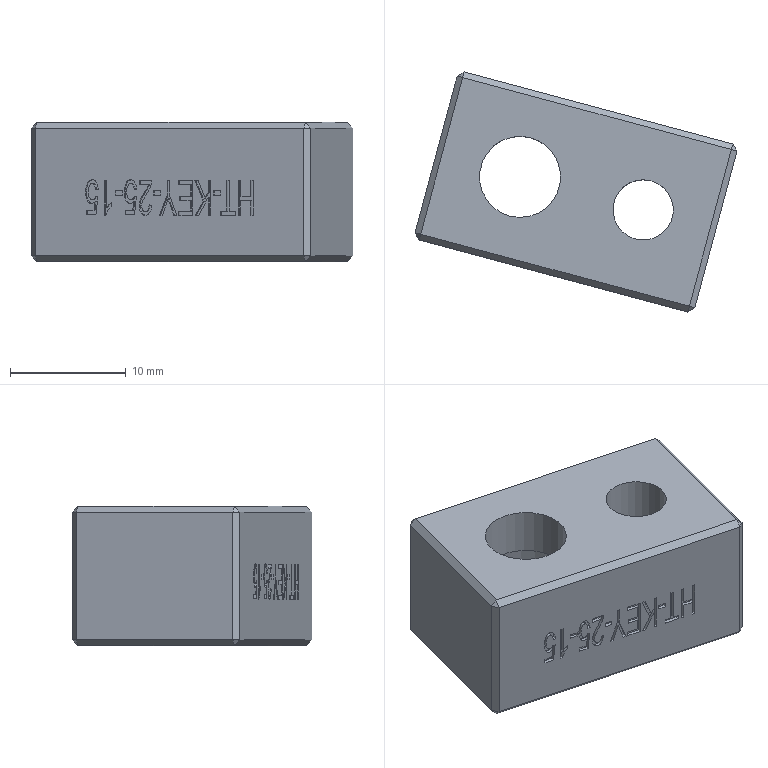Part | NX | features solid 2 | 1 solid | 162 faces | box 27.772 x 20.701 x 12 mm | volume 3198 mm3 | plane 128 | spline 30 | cylinder 4 | commonest cylinder face diameters 7 x2 5.2 x1 11 x1